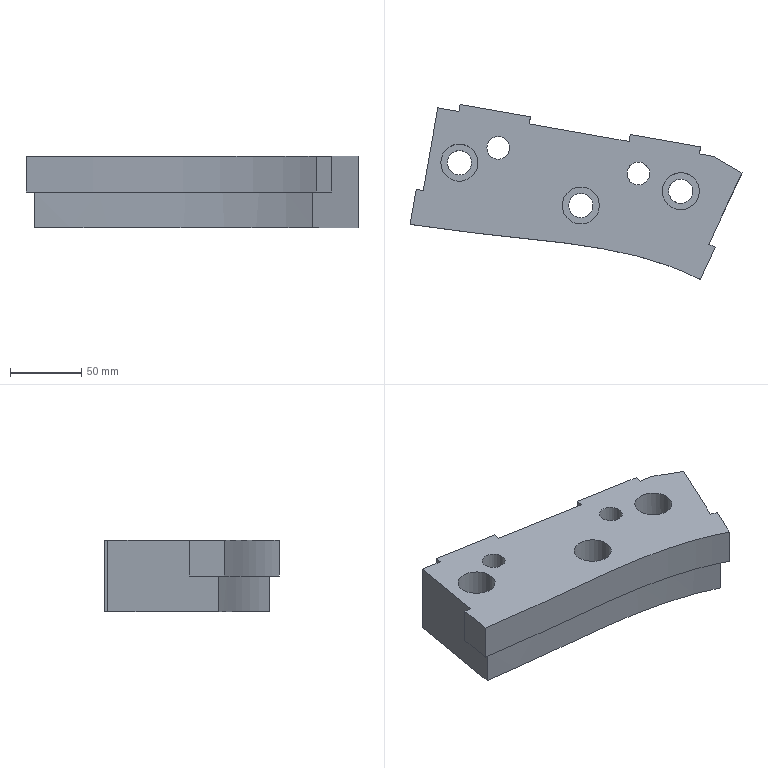Part | NX | features solid 2 | 1 solid | 32 faces | box 232.476 x 122.521 x 50 mm | volume 761001 mm3 | plane 22 | cylinder 8 | spline 2 | commonest cylinder face diameters 17 x3 26 x3 16 x2
STEP:
#1=CARTESIAN_POINT('',(-172.568,-241.894,-25.));
#2=VERTEX_POINT('',#1);
#3=CARTESIAN_POINT('',(-183.133,-264.552,-25.));
#4=VERTEX_POINT('',#3);
#5=CARTESIAN_POINT('',(-183.133,-264.552,-25.));
#6=DIRECTION('',(-0.4226,-0.9063,0.));
#7=VECTOR('',#6,1000.);
#8=LINE('',#5,#7);
#9=EDGE_CURVE('',#2,#4,#8,.T.);
#10=ORIENTED_EDGE('',*,*,#9,.F.);
#11=CARTESIAN_POINT('',(-172.568,-241.894,0.));
#12=VERTEX_POINT('',#11);
#13=CARTESIAN_POINT('',(-172.568,-241.894,-50.));
#14=DIRECTION('',(0.,0.,1.));
#15=VECTOR('',#14,1000.);
#16=LINE('',#13,#15);
#17=EDGE_CURVE('',#2,#12,#16,.T.);
#18=ORIENTED_EDGE('',*,*,#17,.T.);
#19=CARTESIAN_POINT('',(-183.133,-264.552,0.));
#20=VERTEX_POINT('',#19);
#21=CARTESIAN_POINT('',(-183.133,-264.552,0.));
#22=DIRECTION('',(0.4226,0.9063,0.));
#23=VECTOR('',#22,1000.);
#24=LINE('',#21,#23);
#25=EDGE_CURVE('',#20,#12,#24,.T.);
#26=ORIENTED_EDGE('',*,*,#25,.F.);
#27=CARTESIAN_POINT('',(-183.133,-264.552,-50.));
#28=DIRECTION('',(0.,0.,1.));
#29=VECTOR('',#28,1000.);
#30=LINE('',#27,#29);
#31=EDGE_CURVE('',#4,#20,#30,.T.);
#32=ORIENTED_EDGE('',*,*,#31,.F.);
#33=EDGE_LOOP('',(#10,#18,#26,#32));
#34=FACE_BOUND('',#33,.T.);
#35=CARTESIAN_POINT('',(-183.133,-264.552,-50.));
#36=DIRECTION('',(0.9063,-0.4226,0.));
#37=DIRECTION('',(0.4226,0.9063,0.));
#38=AXIS2_PLACEMENT_3D('',#35,#36,#37);
#39=PLANE('',#38);
#40=ADVANCED_FACE('',(#34),#39,.T.);
#41=CARTESIAN_POINT('',(-332.523,-172.421,0.));
#42=VERTEX_POINT('',#41);
#43=CARTESIAN_POINT('',(-324.523,-172.421,0.));
#44=DIRECTION('',(0.,0.,-1.));
#45=DIRECTION('',(-1.,0.,0.));
#46=AXIS2_PLACEMENT_3D('',#43,#44,#45);
#47=CIRCLE('',#46,8.);
#48=EDGE_CURVE('',#42,#42,#47,.T.);
#49=ORIENTED_EDGE('',*,*,#48,.T.);
#50=EDGE_LOOP('',(#49));
#51=FACE_BOUND('',#50,.T.);
#52=CARTESIAN_POINT('',(-234.374,-190.368,0.));
#53=VERTEX_POINT('',#52);
#54=CARTESIAN_POINT('',(-226.374,-190.368,0.));
#55=DIRECTION('',(0.,0.,-1.));
#56=DIRECTION('',(-1.,0.,0.));
#57=AXIS2_PLACEMENT_3D('',#54,#55,#56);
#58=CIRCLE('',#57,8.);
#59=EDGE_CURVE('',#53,#53,#58,.T.);
#60=ORIENTED_EDGE('',*,*,#59,.T.);
#61=EDGE_LOOP('',(#60));
#62=FACE_BOUND('',#61,.T.);
#63=CARTESIAN_POINT('',(-364.729,-182.741,0.));
#64=VERTEX_POINT('',#63);
#65=CARTESIAN_POINT('',(-351.729,-182.741,0.));
#66=DIRECTION('',(0.,0.,-1.));
#67=DIRECTION('',(-1.,0.,0.));
#68=AXIS2_PLACEMENT_3D('',#65,#66,#67);
#69=CIRCLE('',#68,13.);
#70=EDGE_CURVE('',#64,#64,#69,.T.);
#71=ORIENTED_EDGE('',*,*,#70,.T.);
#72=EDGE_LOOP('',(#71));
#73=FACE_BOUND('',#72,.T.);
#74=CARTESIAN_POINT('',(-279.729,-212.741,0.));
#75=VERTEX_POINT('',#74);
#76=CARTESIAN_POINT('',(-266.729,-212.741,0.));
#77=DIRECTION('',(0.,0.,-1.));
#78=DIRECTION('',(-1.,0.,0.));
#79=AXIS2_PLACEMENT_3D('',#76,#77,#78);
#80=CIRCLE('',#79,13.);
#81=EDGE_CURVE('',#75,#75,#80,.T.);
#82=ORIENTED_EDGE('',*,*,#81,.T.);
#83=EDGE_LOOP('',(#82));
#84=FACE_BOUND('',#83,.T.);
#85=CARTESIAN_POINT('',(-209.729,-202.741,0.));
#86=VERTEX_POINT('',#85);
#87=CARTESIAN_POINT('',(-196.729,-202.741,0.));
#88=DIRECTION('',(0.,0.,-1.));
#89=DIRECTION('',(-1.,0.,0.));
#90=AXIS2_PLACEMENT_3D('',#87,#88,#89);
#91=CIRCLE('',#90,13.);
#92=EDGE_CURVE('',#86,#86,#91,.T.);
#93=ORIENTED_EDGE('',*,*,#92,.T.);
#94=EDGE_LOOP('',(#93));
#95=FACE_BOUND('',#94,.T.);
#96=CARTESIAN_POINT('',(-177.099,-239.781,0.));
#97=VERTEX_POINT('',#96);
#98=CARTESIAN_POINT('',(-177.099,-239.781,0.));
#99=DIRECTION('',(0.9063,-0.4226,0.));
#100=VECTOR('',#99,1000.);
#101=LINE('',#98,#100);
#102=EDGE_CURVE('',#97,#12,#101,.T.);
#103=ORIENTED_EDGE('',*,*,#102,.F.);
#104=CARTESIAN_POINT('',(-153.848,-189.919,0.));
#105=VERTEX_POINT('',#104);
#106=CARTESIAN_POINT('',(-187.665,-262.438,0.));
#107=DIRECTION('',(0.4226,0.9063,0.));
#108=VECTOR('',#107,1000.);
#109=LINE('',#106,#108);
#110=EDGE_CURVE('',#97,#105,#109,.T.);
#111=ORIENTED_EDGE('',*,*,#110,.T.);
#112=CARTESIAN_POINT('',(-173.828,-178.383,0.));
#113=VERTEX_POINT('',#112);
#114=CARTESIAN_POINT('',(-229.835,-146.048,0.));
#115=DIRECTION('',(0.866,-0.5,0.));
#116=VECTOR('',#115,1000.);
#117=LINE('',#114,#116);
#118=EDGE_CURVE('',#113,#105,#117,.T.);
#119=ORIENTED_EDGE('',*,*,#118,.F.);
#120=CARTESIAN_POINT('',(-183.676,-176.647,0.));
#121=VERTEX_POINT('',#120);
#122=CARTESIAN_POINT('',(-371.767,-143.481,0.));
#123=DIRECTION('',(0.9848,-0.1736,0.));
#124=VECTOR('',#123,1000.);
#125=LINE('',#122,#124);
#126=EDGE_CURVE('',#121,#113,#125,.T.);
#127=ORIENTED_EDGE('',*,*,#126,.F.);
#128=CARTESIAN_POINT('',(-182.808,-171.723,0.));
#129=VERTEX_POINT('',#128);
#130=CARTESIAN_POINT('',(-183.676,-176.647,0.));
#131=DIRECTION('',(0.1736,0.9848,0.));
#132=VECTOR('',#131,1000.);
#133=LINE('',#130,#132);
#134=EDGE_CURVE('',#121,#129,#133,.T.);
#135=ORIENTED_EDGE('',*,*,#134,.T.);
#136=CARTESIAN_POINT('',(-232.048,-163.04,0.));
#137=VERTEX_POINT('',#136);
#138=CARTESIAN_POINT('',(-370.899,-138.557,0.));
#139=DIRECTION('',(0.9848,-0.1736,0.));
#140=VECTOR('',#139,1000.);
#141=LINE('',#138,#140);
#142=EDGE_CURVE('',#137,#129,#141,.T.);
#143=ORIENTED_EDGE('',*,*,#142,.F.);
#144=CARTESIAN_POINT('',(-232.916,-167.964,0.));
#145=VERTEX_POINT('',#144);
#146=CARTESIAN_POINT('',(-232.916,-167.964,0.));
#147=DIRECTION('',(0.1736,0.9848,0.));
#148=VECTOR('',#147,1000.);
#149=LINE('',#146,#148);
#150=EDGE_CURVE('',#145,#137,#149,.T.);
#151=ORIENTED_EDGE('',*,*,#150,.F.);
#152=CARTESIAN_POINT('',(-302.831,-155.637,0.));
#153=VERTEX_POINT('',#152);
#154=CARTESIAN_POINT('',(-371.767,-143.481,0.));
#155=DIRECTION('',(0.9848,-0.1736,0.));
#156=VECTOR('',#155,1000.);
#157=LINE('',#154,#156);
#158=EDGE_CURVE('',#153,#145,#157,.T.);
#159=ORIENTED_EDGE('',*,*,#158,.F.);
#160=CARTESIAN_POINT('',(-301.962,-150.713,0.));
#161=VERTEX_POINT('',#160);
#162=CARTESIAN_POINT('',(-302.831,-155.637,0.));
#163=DIRECTION('',(0.1736,0.9848,0.));
#164=VECTOR('',#163,1000.);
#165=LINE('',#162,#164);
#166=EDGE_CURVE('',#153,#161,#165,.T.);
#167=ORIENTED_EDGE('',*,*,#166,.T.);
#168=CARTESIAN_POINT('',(-351.203,-142.03,0.));
#169=VERTEX_POINT('',#168);
#170=CARTESIAN_POINT('',(-504.826,-114.942,0.));
#171=DIRECTION('',(0.9848,-0.1736,0.));
#172=VECTOR('',#171,1000.);
#173=LINE('',#170,#172);
#174=EDGE_CURVE('',#169,#161,#173,.T.);
#175=ORIENTED_EDGE('',*,*,#174,.F.);
#176=CARTESIAN_POINT('',(-352.071,-146.954,0.));
#177=VERTEX_POINT('',#176);
#178=CARTESIAN_POINT('',(-352.071,-146.954,0.));
#179=DIRECTION('',(0.1736,0.9848,0.));
#180=VECTOR('',#179,1000.);
#181=LINE('',#178,#180);
#182=EDGE_CURVE('',#177,#169,#181,.T.);
#183=ORIENTED_EDGE('',*,*,#182,.F.);
#184=CARTESIAN_POINT('',(-366.843,-144.35,0.));
#185=VERTEX_POINT('',#184);
#186=CARTESIAN_POINT('',(-371.767,-143.481,0.));
#187=DIRECTION('',(0.9848,-0.1736,0.));
#188=VECTOR('',#187,1000.);
#189=LINE('',#186,#188);
#190=EDGE_CURVE('',#185,#177,#189,.T.);
#191=ORIENTED_EDGE('',*,*,#190,.F.);
#192=CARTESIAN_POINT('',(-377.059,-202.288,0.));
#193=VERTEX_POINT('',#192);
#194=CARTESIAN_POINT('',(-381.401,-226.908,0.));
#195=DIRECTION('',(0.1736,0.9848,0.));
#196=VECTOR('',#195,1000.);
#197=LINE('',#194,#196);
#198=EDGE_CURVE('',#193,#185,#197,.T.);
#199=ORIENTED_EDGE('',*,*,#198,.F.);
#200=CARTESIAN_POINT('',(-381.983,-201.42,0.));
#201=VERTEX_POINT('',#200);
#202=CARTESIAN_POINT('',(-377.059,-202.288,0.));
#203=DIRECTION('',(-0.9848,0.1736,0.));
#204=VECTOR('',#203,1000.);
#205=LINE('',#202,#204);
#206=EDGE_CURVE('',#193,#201,#205,.T.);
#207=ORIENTED_EDGE('',*,*,#206,.T.);
#208=CARTESIAN_POINT('',(-386.325,-226.04,0.));
#209=VERTEX_POINT('',#208);
#210=CARTESIAN_POINT('',(-386.325,-226.04,0.));
#211=DIRECTION('',(0.1736,0.9848,0.));
#212=VECTOR('',#211,1000.);
#213=LINE('',#210,#212);
#214=EDGE_CURVE('',#209,#201,#213,.T.);
#215=ORIENTED_EDGE('',*,*,#214,.F.);
#216=CARTESIAN_POINT('',(-386.325,-226.04,0.));
#217=CARTESIAN_POINT('',(-385.988,-226.092,0.));
#218=CARTESIAN_POINT('',(-371.935,-228.253,0.));
#219=CARTESIAN_POINT('',(-344.075,-231.948,0.));
#220=CARTESIAN_POINT('',(-302.639,-236.064,0.));
#221=CARTESIAN_POINT('',(-261.264,-240.795,0.));
#222=CARTESIAN_POINT('',(-220.785,-248.799,0.));
#223=CARTESIAN_POINT('',(-195.074,-258.417,0.));
#224=CARTESIAN_POINT('',(-183.133,-264.552,0.));
#225=B_SPLINE_CURVE_WITH_KNOTS('',3,(#216,#217,#218,#219,#220,#221,#222,#223,#224),.UNSPECIFIED.,.F.,.F.,(4,1,1,1,1,1,4),(0.,0.004908,0.2052,0.4055,0.6058,0.8062,1.),.UNSPECIFIED.);
#226=EDGE_CURVE('',#209,#20,#225,.T.);
#227=ORIENTED_EDGE('',*,*,#226,.T.);
#228=ORIENTED_EDGE('',*,*,#25,.T.);
#229=EDGE_LOOP('',(#103,#111,#119,#127,#135,#143,#151,#159,#167,#175,#183,#191,#199,#207,#215,#227,#228));
#230=FACE_BOUND('',#229,.T.);
#231=CARTESIAN_POINT('',(-283.137,-238.369,0.));
#232=DIRECTION('',(0.,0.,-1.));
#233=DIRECTION('',(-1.,0.,0.));
#234=AXIS2_PLACEMENT_3D('',#231,#232,#233);
#235=PLANE('',#234);
#236=ADVANCED_FACE('',(#51,#62,#73,#84,#95,#230),#235,.F.);
#237=CARTESIAN_POINT('',(-177.099,-239.781,-25.));
#238=VERTEX_POINT('',#237);
#239=CARTESIAN_POINT('',(-177.099,-239.781,-25.));
#240=DIRECTION('',(0.9063,-0.4226,0.));
#241=VECTOR('',#240,1000.);
#242=LINE('',#239,#241);
#243=EDGE_CURVE('',#238,#2,#242,.T.);
#244=ORIENTED_EDGE('',*,*,#243,.T.);
#245=ORIENTED_EDGE('',*,*,#9,.T.);
#246=CARTESIAN_POINT('',(-386.325,-226.04,-25.));
#247=VERTEX_POINT('',#246);
#248=CARTESIAN_POINT('',(-386.325,-226.04,-25.));
#249=CARTESIAN_POINT('',(-385.988,-226.092,-25.));
#250=CARTESIAN_POINT('',(-371.935,-228.253,-25.));
#251=CARTESIAN_POINT('',(-344.075,-231.948,-25.));
#252=CARTESIAN_POINT('',(-302.639,-236.064,-25.));
#253=CARTESIAN_POINT('',(-261.264,-240.795,-25.));
#254=CARTESIAN_POINT('',(-220.785,-248.799,-25.));
#255=CARTESIAN_POINT('',(-195.074,-258.417,-25.));
#256=CARTESIAN_POINT('',(-183.133,-264.552,-25.));
#257=B_SPLINE_CURVE_WITH_KNOTS('',3,(#248,#249,#250,#251,#252,#253,#254,#255,#256),.UNSPECIFIED.,.F.,.F.,(4,1,1,1,1,1,4),(0.,0.004908,0.2052,0.4055,0.6058,0.8062,1.),.UNSPECIFIED.);
#258=EDGE_CURVE('',#4,#247,#257,.F.);
#259=ORIENTED_EDGE('',*,*,#258,.T.);
#260=CARTESIAN_POINT('',(-381.983,-201.42,-25.));
#261=VERTEX_POINT('',#260);
#262=CARTESIAN_POINT('',(-386.325,-226.04,-25.));
#263=DIRECTION('',(-0.1736,-0.9848,0.));
#264=VECTOR('',#263,1000.);
#265=LINE('',#262,#264);
#266=EDGE_CURVE('',#261,#247,#265,.T.);
#267=ORIENTED_EDGE('',*,*,#266,.F.);
#268=CARTESIAN_POINT('',(-377.059,-202.288,-25.));
#269=VERTEX_POINT('',#268);
#270=CARTESIAN_POINT('',(-377.059,-202.288,-25.));
#271=DIRECTION('',(-0.9848,0.1736,0.));
#272=VECTOR('',#271,1000.);
#273=LINE('',#270,#272);
#274=EDGE_CURVE('',#269,#261,#273,.T.);
#275=ORIENTED_EDGE('',*,*,#274,.F.);
#276=CARTESIAN_POINT('',(-380.511,-221.865,-25.));
#277=VERTEX_POINT('',#276);
#278=CARTESIAN_POINT('',(-381.401,-226.908,-25.));
#279=DIRECTION('',(-0.1736,-0.9848,0.));
#280=VECTOR('',#279,1000.);
#281=LINE('',#278,#280);
#282=EDGE_CURVE('',#277,#269,#281,.F.);
#283=ORIENTED_EDGE('',*,*,#282,.F.);
#284=CARTESIAN_POINT('',(-185.501,-257.798,-25.));
#285=VERTEX_POINT('',#284);
#286=CARTESIAN_POINT('',(-380.511,-221.865,-25.));
#287=CARTESIAN_POINT('',(-364.297,-224.285,-25.));
#288=CARTESIAN_POINT('',(-331.761,-228.294,-25.));
#289=CARTESIAN_POINT('',(-282.53,-232.98,-25.));
#290=CARTESIAN_POINT('',(-233.079,-240.247,-25.));
#291=CARTESIAN_POINT('',(-200.769,-250.502,-25.));
#292=CARTESIAN_POINT('',(-185.501,-257.798,-25.));
#293=B_SPLINE_CURVE_WITH_KNOTS('',3,(#286,#287,#288,#289,#290,#291,#292),.UNSPECIFIED.,.F.,.F.,(4,1,1,1,4),(0.0247,0.2624,0.5002,0.7379,0.9757),.UNSPECIFIED.);
#294=EDGE_CURVE('',#277,#285,#293,.T.);
#295=ORIENTED_EDGE('',*,*,#294,.T.);
#296=CARTESIAN_POINT('',(-187.665,-262.438,-25.));
#297=DIRECTION('',(-0.4226,-0.9063,0.));
#298=VECTOR('',#297,1000.);
#299=LINE('',#296,#298);
#300=EDGE_CURVE('',#285,#238,#299,.F.);
#301=ORIENTED_EDGE('',*,*,#300,.T.);
#302=EDGE_LOOP('',(#244,#245,#259,#267,#275,#283,#295,#301));
#303=FACE_BOUND('',#302,.T.);
#304=CARTESIAN_POINT('',(-386.325,-226.04,-25.));
#305=DIRECTION('',(0.,0.,1.));
#306=DIRECTION('',(1.,0.,0.));
#307=AXIS2_PLACEMENT_3D('',#304,#305,#306);
#308=PLANE('',#307);
#309=ADVANCED_FACE('',(#303),#308,.F.);
#310=ORIENTED_EDGE('',*,*,#118,.T.);
#311=CARTESIAN_POINT('',(-153.848,-189.919,-50.));
#312=VERTEX_POINT('',#311);
#313=CARTESIAN_POINT('',(-153.848,-189.919,-25.));
#314=DIRECTION('',(0.,0.,-1.));
#315=VECTOR('',#314,1000.);
#316=LINE('',#313,#315);
#317=EDGE_CURVE('',#105,#312,#316,.T.);
#318=ORIENTED_EDGE('',*,*,#317,.T.);
#319=CARTESIAN_POINT('',(-173.828,-178.383,-50.));
#320=VERTEX_POINT('',#319);
#321=CARTESIAN_POINT('',(-229.835,-146.048,-50.));
#322=DIRECTION('',(0.866,-0.5,0.));
#323=VECTOR('',#322,1000.);
#324=LINE('',#321,#323);
#325=EDGE_CURVE('',#320,#312,#324,.T.);
#326=ORIENTED_EDGE('',*,*,#325,.F.);
#327=CARTESIAN_POINT('',(-173.828,-178.383,-50.));
#328=DIRECTION('',(0.,0.,1.));
#329=VECTOR('',#328,1000.);
#330=LINE('',#327,#329);
#331=EDGE_CURVE('',#320,#113,#330,.T.);
#332=ORIENTED_EDGE('',*,*,#331,.T.);
#333=EDGE_LOOP('',(#310,#318,#326,#332));
#334=FACE_BOUND('',#333,.T.);
#335=CARTESIAN_POINT('',(32.129,-297.293,0.));
#336=DIRECTION('',(0.5,0.866,0.));
#337=DIRECTION('',(-0.866,0.5,0.));
#338=AXIS2_PLACEMENT_3D('',#335,#336,#337);
#339=PLANE('',#338);
#340=ADVANCED_FACE('',(#334),#339,.T.);
#341=CARTESIAN_POINT('',(-302.831,-155.637,-50.));
#342=VERTEX_POINT('',#341);
#343=CARTESIAN_POINT('',(-302.831,-155.637,-50.));
#344=DIRECTION('',(0.,0.,1.));
#345=VECTOR('',#344,1000.);
#346=LINE('',#343,#345);
#347=EDGE_CURVE('',#342,#153,#346,.T.);
#348=ORIENTED_EDGE('',*,*,#347,.T.);
#349=ORIENTED_EDGE('',*,*,#158,.T.);
#350=CARTESIAN_POINT('',(-232.916,-167.964,-50.));
#351=VERTEX_POINT('',#350);
#352=CARTESIAN_POINT('',(-232.916,-167.964,-50.));
#353=DIRECTION('',(0.,0.,-1.));
#354=VECTOR('',#353,1000.);
#355=LINE('',#352,#354);
#356=EDGE_CURVE('',#145,#351,#355,.T.);
#357=ORIENTED_EDGE('',*,*,#356,.T.);
#358=CARTESIAN_POINT('',(-371.767,-143.481,-50.));
#359=DIRECTION('',(0.9848,-0.1736,0.));
#360=VECTOR('',#359,1000.);
#361=LINE('',#358,#360);
#362=EDGE_CURVE('',#342,#351,#361,.T.);
#363=ORIENTED_EDGE('',*,*,#362,.F.);
#364=EDGE_LOOP('',(#348,#349,#357,#363));
#365=FACE_BOUND('',#364,.T.);
#366=CARTESIAN_POINT('',(-371.767,-143.481,-50.));
#367=DIRECTION('',(-0.1736,-0.9848,0.));
#368=DIRECTION('',(0.9848,-0.1736,0.));
#369=AXIS2_PLACEMENT_3D('',#366,#367,#368);
#370=PLANE('',#369);
#371=ADVANCED_FACE('',(#365),#370,.F.);
#372=CARTESIAN_POINT('',(-366.843,-144.35,-50.));
#373=VERTEX_POINT('',#372);
#374=CARTESIAN_POINT('',(-366.843,-144.35,-50.));
#375=DIRECTION('',(0.,0.,-1.));
#376=VECTOR('',#375,1000.);
#377=LINE('',#374,#376);
#378=EDGE_CURVE('',#185,#373,#377,.T.);
#379=ORIENTED_EDGE('',*,*,#378,.F.);
#380=ORIENTED_EDGE('',*,*,#190,.T.);
#381=CARTESIAN_POINT('',(-352.071,-146.954,-50.));
#382=VERTEX_POINT('',#381);
#383=CARTESIAN_POINT('',(-352.071,-146.954,-50.));
#384=DIRECTION('',(0.,0.,-1.));
#385=VECTOR('',#384,1000.);
#386=LINE('',#383,#385);
#387=EDGE_CURVE('',#177,#382,#386,.T.);
#388=ORIENTED_EDGE('',*,*,#387,.T.);
#389=CARTESIAN_POINT('',(-371.767,-143.481,-50.));
#390=DIRECTION('',(0.9848,-0.1736,0.));
#391=VECTOR('',#390,1000.);
#392=LINE('',#389,#391);
#393=EDGE_CURVE('',#373,#382,#392,.T.);
#394=ORIENTED_EDGE('',*,*,#393,.F.);
#395=EDGE_LOOP('',(#379,#380,#388,#394));
#396=FACE_BOUND('',#395,.T.);
#397=CARTESIAN_POINT('',(-371.767,-143.481,-50.));
#398=DIRECTION('',(-0.1736,-0.9848,0.));
#399=DIRECTION('',(0.9848,-0.1736,0.));
#400=AXIS2_PLACEMENT_3D('',#397,#398,#399);
#401=PLANE('',#400);
#402=ADVANCED_FACE('',(#396),#401,.F.);
#403=CARTESIAN_POINT('',(-183.676,-176.647,-50.));
#404=VERTEX_POINT('',#403);
#405=CARTESIAN_POINT('',(-183.676,-176.647,-50.));
#406=DIRECTION('',(0.,0.,1.));
#407=VECTOR('',#406,1000.);
#408=LINE('',#405,#407);
#409=EDGE_CURVE('',#404,#121,#408,.T.);
#410=ORIENTED_EDGE('',*,*,#409,.T.);
#411=ORIENTED_EDGE('',*,*,#126,.T.);
#412=ORIENTED_EDGE('',*,*,#331,.F.);
#413=CARTESIAN_POINT('',(-371.767,-143.481,-50.));
#414=DIRECTION('',(0.9848,-0.1736,0.));
#415=VECTOR('',#414,1000.);
#416=LINE('',#413,#415);
#417=EDGE_CURVE('',#404,#320,#416,.T.);
#418=ORIENTED_EDGE('',*,*,#417,.F.);
#419=EDGE_LOOP('',(#410,#411,#412,#418));
#420=FACE_BOUND('',#419,.T.);
#421=CARTESIAN_POINT('',(-371.767,-143.481,-50.));
#422=DIRECTION('',(-0.1736,-0.9848,0.));
#423=DIRECTION('',(0.9848,-0.1736,0.));
#424=AXIS2_PLACEMENT_3D('',#421,#422,#423);
#425=PLANE('',#424);
#426=ADVANCED_FACE('',(#420),#425,.F.);
#427=CARTESIAN_POINT('',(-332.523,-172.421,-50.));
#428=VERTEX_POINT('',#427);
#429=CARTESIAN_POINT('',(-324.523,-172.421,-50.));
#430=DIRECTION('',(0.,0.,-1.));
#431=DIRECTION('',(-1.,0.,0.));
#432=AXIS2_PLACEMENT_3D('',#429,#430,#431);
#433=CIRCLE('',#432,8.);
#434=EDGE_CURVE('',#428,#428,#433,.T.);
#435=ORIENTED_EDGE('',*,*,#434,.F.);
#436=EDGE_LOOP('',(#435));
#437=FACE_BOUND('',#436,.T.);
#438=CARTESIAN_POINT('',(-234.374,-190.368,-50.));
#439=VERTEX_POINT('',#438);
#440=CARTESIAN_POINT('',(-226.374,-190.368,-50.));
#441=DIRECTION('',(0.,0.,-1.));
#442=DIRECTION('',(-1.,0.,0.));
#443=AXIS2_PLACEMENT_3D('',#440,#441,#442);
#444=CIRCLE('',#443,8.);
#445=EDGE_CURVE('',#439,#439,#444,.T.);
#446=ORIENTED_EDGE('',*,*,#445,.F.);
#447=EDGE_LOOP('',(#446));
#448=FACE_BOUND('',#447,.T.);
#449=CARTESIAN_POINT('',(-205.229,-202.741,-50.));
#450=VERTEX_POINT('',#449);
#451=CARTESIAN_POINT('',(-196.729,-202.741,-50.));
#452=DIRECTION('',(0.,0.,-1.));
#453=DIRECTION('',(-1.,0.,0.));
#454=AXIS2_PLACEMENT_3D('',#451,#452,#453);
#455=CIRCLE('',#454,8.5);
#456=EDGE_CURVE('',#450,#450,#455,.T.);
#457=ORIENTED_EDGE('',*,*,#456,.F.);
#458=EDGE_LOOP('',(#457));
#459=FACE_BOUND('',#458,.T.);
#460=CARTESIAN_POINT('',(-275.229,-212.741,-50.));
#461=VERTEX_POINT('',#460);
#462=CARTESIAN_POINT('',(-266.729,-212.741,-50.));
#463=DIRECTION('',(0.,0.,-1.));
#464=DIRECTION('',(-1.,0.,0.));
#465=AXIS2_PLACEMENT_3D('',#462,#463,#464);
#466=CIRCLE('',#465,8.5);
#467=EDGE_CURVE('',#461,#461,#466,.T.);
#468=ORIENTED_EDGE('',*,*,#467,.F.);
#469=EDGE_LOOP('',(#468));
#470=FACE_BOUND('',#469,.T.);
#471=CARTESIAN_POINT('',(-360.229,-182.741,-50.));
#472=VERTEX_POINT('',#471);
#473=CARTESIAN_POINT('',(-351.729,-182.741,-50.));
#474=DIRECTION('',(0.,0.,-1.));
#475=DIRECTION('',(-1.,0.,0.));
#476=AXIS2_PLACEMENT_3D('',#473,#474,#475);
#477=CIRCLE('',#476,8.5);
#478=EDGE_CURVE('',#472,#472,#477,.T.);
#479=ORIENTED_EDGE('',*,*,#478,.F.);
#480=EDGE_LOOP('',(#479));
#481=FACE_BOUND('',#480,.T.);
#482=ORIENTED_EDGE('',*,*,#393,.T.);
#483=CARTESIAN_POINT('',(-351.203,-142.03,-50.));
#484=VERTEX_POINT('',#483);
#485=CARTESIAN_POINT('',(-352.071,-146.954,-50.));
#486=DIRECTION('',(0.1736,0.9848,0.));
#487=VECTOR('',#486,1000.);
#488=LINE('',#485,#487);
#489=EDGE_CURVE('',#382,#484,#488,.T.);
#490=ORIENTED_EDGE('',*,*,#489,.T.);
#491=CARTESIAN_POINT('',(-301.962,-150.713,-50.));
#492=VERTEX_POINT('',#491);
#493=CARTESIAN_POINT('',(-504.826,-114.942,-50.));
#494=DIRECTION('',(0.9848,-0.1736,0.));
#495=VECTOR('',#494,1000.);
#496=LINE('',#493,#495);
#497=EDGE_CURVE('',#484,#492,#496,.T.);
#498=ORIENTED_EDGE('',*,*,#497,.T.);
#499=CARTESIAN_POINT('',(-302.831,-155.637,-50.));
#500=DIRECTION('',(0.1736,0.9848,0.));
#501=VECTOR('',#500,1000.);
#502=LINE('',#499,#501);
#503=EDGE_CURVE('',#342,#492,#502,.T.);
#504=ORIENTED_EDGE('',*,*,#503,.F.);
#505=ORIENTED_EDGE('',*,*,#362,.T.);
#506=CARTESIAN_POINT('',(-232.048,-163.04,-50.));
#507=VERTEX_POINT('',#506);
#508=CARTESIAN_POINT('',(-232.916,-167.964,-50.));
#509=DIRECTION('',(0.1736,0.9848,0.));
#510=VECTOR('',#509,1000.);
#511=LINE('',#508,#510);
#512=EDGE_CURVE('',#351,#507,#511,.T.);
#513=ORIENTED_EDGE('',*,*,#512,.T.);
#514=CARTESIAN_POINT('',(-182.808,-171.723,-50.));
#515=VERTEX_POINT('',#514);
#516=CARTESIAN_POINT('',(-370.899,-138.557,-50.));
#517=DIRECTION('',(0.9848,-0.1736,0.));
#518=VECTOR('',#517,1000.);
#519=LINE('',#516,#518);
#520=EDGE_CURVE('',#507,#515,#519,.T.);
#521=ORIENTED_EDGE('',*,*,#520,.T.);
#522=CARTESIAN_POINT('',(-183.676,-176.647,-50.));
#523=DIRECTION('',(0.1736,0.9848,0.));
#524=VECTOR('',#523,1000.);
#525=LINE('',#522,#524);
#526=EDGE_CURVE('',#404,#515,#525,.T.);
#527=ORIENTED_EDGE('',*,*,#526,.F.);
#528=ORIENTED_EDGE('',*,*,#417,.T.);
#529=ORIENTED_EDGE('',*,*,#325,.T.);
#530=CARTESIAN_POINT('',(-185.501,-257.798,-50.));
#531=VERTEX_POINT('',#530);
#532=CARTESIAN_POINT('',(-195.498,-279.236,-50.));
#533=DIRECTION('',(0.4226,0.9063,0.));
#534=VECTOR('',#533,1000.);
#535=LINE('',#532,#534);
#536=EDGE_CURVE('',#531,#312,#535,.T.);
#537=ORIENTED_EDGE('',*,*,#536,.F.);
#538=CARTESIAN_POINT('',(-380.511,-221.865,-50.));
#539=VERTEX_POINT('',#538);
#540=CARTESIAN_POINT('',(-185.501,-257.798,-50.));
#541=CARTESIAN_POINT('',(-188.943,-256.153,-50.));
#542=CARTESIAN_POINT('',(-196.057,-253.02,-50.));
#543=CARTESIAN_POINT('',(-205.525,-249.494,-50.));
#544=CARTESIAN_POINT('',(-213.444,-246.908,-50.));
#545=CARTESIAN_POINT('',(-219.56,-245.085,-50.));
#546=CARTESIAN_POINT('',(-224.788,-243.666,-50.));
#547=CARTESIAN_POINT('',(-228.548,-242.719,-50.));
#548=CARTESIAN_POINT('',(-230.68,-242.201,-50.));
#549=CARTESIAN_POINT('',(-232.396,-241.795,-50.));
#550=CARTESIAN_POINT('',(-233.719,-241.49,-50.));
#551=CARTESIAN_POINT('',(-235.645,-241.054,-50.));
#552=CARTESIAN_POINT('',(-239.001,-240.319,-50.));
#553=CARTESIAN_POINT('',(-243.982,-239.298,-50.));
#554=CARTESIAN_POINT('',(-249.135,-238.331,-50.));
#555=CARTESIAN_POINT('',(-252.875,-237.675,-50.));
#556=CARTESIAN_POINT('',(-255.001,-237.314,-50.));
#557=CARTESIAN_POINT('',(-256.723,-237.029,-50.));
#558=CARTESIAN_POINT('',(-258.029,-236.817,-50.));
#559=CARTESIAN_POINT('',(-259.948,-236.511,-50.));
#560=CARTESIAN_POINT('',(-263.303,-235.991,-50.));
#561=CARTESIAN_POINT('',(-267.323,-235.401,-50.));
#562=CARTESIAN_POINT('',(-271.486,-234.824,-50.));
#563=CARTESIAN_POINT('',(-274.691,-234.394,-50.));
#564=CARTESIAN_POINT('',(-277.413,-234.042,-50.));
#565=CARTESIAN_POINT('',(-279.378,-233.794,-50.));
#566=CARTESIAN_POINT('',(-280.471,-233.658,-50.));
#567=CARTESIAN_POINT('',(-281.408,-233.543,-50.));
#568=CARTESIAN_POINT('',(-281.919,-233.481,-50.));
#569=CARTESIAN_POINT('',(-282.768,-233.377,-50.));
#570=CARTESIAN_POINT('',(-284.222,-233.202,-50.));
#571=CARTESIAN_POINT('',(-286.447,-232.939,-50.));
#572=CARTESIAN_POINT('',(-289.279,-232.612,-50.));
#573=CARTESIAN_POINT('',(-292.293,-232.271,-50.));
#574=CARTESIAN_POINT('',(-295.483,-231.916,-50.));
#575=CARTESIAN_POINT('',(-298.29,-231.609,-50.));
#576=CARTESIAN_POINT('',(-300.624,-231.356,-50.));
#577=CARTESIAN_POINT('',(-302.12,-231.195,-50.));
#578=CARTESIAN_POINT('',(-303.338,-231.065,-50.));
#579=CARTESIAN_POINT('',(-304.266,-230.967,-50.));
#580=CARTESIAN_POINT('',(-305.039,-230.885,-50.));
#581=CARTESIAN_POINT('',(-305.604,-230.825,-50.));
#582=CARTESIAN_POINT('',(-305.897,-230.794,-50.));
#583=CARTESIAN_POINT('',(-306.206,-230.761,-50.));
#584=CARTESIAN_POINT('',(-306.179,-230.764,-50.));
#585=CARTESIAN_POINT('',(-306.269,-230.754,-50.));
#586=CARTESIAN_POINT('',(-306.387,-230.742,-50.));
#587=CARTESIAN_POINT('',(-306.631,-230.716,-50.));
#588=CARTESIAN_POINT('',(-306.988,-230.679,-50.));
#589=CARTESIAN_POINT('',(-307.569,-230.618,-50.));
#590=CARTESIAN_POINT('',(-308.484,-230.522,-50.));
#591=CARTESIAN_POINT('',(-309.885,-230.375,-50.));
#592=CARTESIAN_POINT('',(-311.587,-230.197,-50.));
#593=CARTESIAN_POINT('',(-313.597,-229.986,-50.));
#594=CARTESIAN_POINT('',(-315.512,-229.786,-50.));
#595=CARTESIAN_POINT('',(-317.008,-229.629,-50.));
#596=CARTESIAN_POINT('',(-317.865,-229.539,-50.));
#597=CARTESIAN_POINT('',(-318.629,-229.459,-50.));
#598=CARTESIAN_POINT('',(-319.019,-229.419,-50.));
#599=CARTESIAN_POINT('',(-319.661,-229.351,-50.));
#600=CARTESIAN_POINT('',(-320.707,-229.242,-50.));
#601=CARTESIAN_POINT('',(-322.181,-229.087,-50.));
#602=CARTESIAN_POINT('',(-323.854,-228.91,-50.));
#603=CARTESIAN_POINT('',(-325.448,-228.741,-50.));
#604=CARTESIAN_POINT('',(-326.957,-228.581,-50.));
#605=CARTESIAN_POINT('',(-328.39,-228.428,-50.));
#606=CARTESIAN_POINT('',(-329.497,-228.31,-50.));
#607=CARTESIAN_POINT('',(-330.382,-228.214,-50.));
#608=CARTESIAN_POINT('',(-330.914,-228.157,-50.));
#609=CARTESIAN_POINT('',(-331.852,-228.055,-50.));
#610=CARTESIAN_POINT('',(-332.948,-227.936,-50.));
#611=CARTESIAN_POINT('',(-334.908,-227.722,-50.));
#612=CARTESIAN_POINT('',(-337.597,-227.424,-50.));
#613=CARTESIAN_POINT('',(-340.724,-227.071,-50.));
#614=CARTESIAN_POINT('',(-343.715,-226.728,-50.));
#615=CARTESIAN_POINT('',(-345.905,-226.471,-50.));
#616=CARTESIAN_POINT('',(-347.273,-226.308,-50.));
#617=CARTESIAN_POINT('',(-348.307,-226.185,-50.));
#618=CARTESIAN_POINT('',(-350.179,-225.96,-50.));
#619=CARTESIAN_POINT('',(-352.808,-225.638,-50.));
#620=CARTESIAN_POINT('',(-357.009,-225.113,-50.));
#621=CARTESIAN_POINT('',(-362.211,-224.441,-50.));
#622=CARTESIAN_POINT('',(-370.443,-223.332,-50.));
#623=CARTESIAN_POINT('',(-376.512,-222.462,-50.));
#624=CARTESIAN_POINT('',(-380.511,-221.865,-50.));
#625=B_SPLINE_CURVE_WITH_KNOTS('',3,(#540,#541,#542,#543,#544,#545,#546,#547,#548,#549,#550,#551,#552,#553,#554,#555,#556,#557,#558,#559,#560,#561,#562,#563,#564,#565,#566,#567,#568,#569,#570,#571,#572,#573,#574,#575,#576,#577,#578,#579,#580,#581,#582,#583,#584,#585,#586,#587,#588,#589,#590,#591,#592,#593,#594,#595,#596,#597,#598,#599,#600,#601,#602,#603,#604,#605,#606,#607,#608,#609,#610,#611,#612,#613,#614,#615,#616,#617,#618,#619,#620,#621,#622,#623,#624),.UNSPECIFIED.,.F.,.F.,(4,1,1,1,1,1,1,1,1,1,1,1,1,1,1,1,1,1,1,1,1,1,1,1,1,1,1,1,1,1,1,1,1,1,1,1,1,1,1,1,1,1,1,1,1,1,1,1,1,1,1,1,1,1,1,1,1,1,1,1,1,1,1,1,1,1,1,1,1,1,1,1,1,1,1,1,1,1,1,1,1,1,4),(0.,0.0625,0.125,0.1562,0.1875,0.2188,0.2344,0.2422,0.25,0.2578,0.2656,0.2812,0.3125,0.3438,0.3594,0.3672,0.375,0.3828,0.3906,0.4062,0.4375,0.4531,0.4688,0.4844,0.4922,0.4961,0.5,0.5039,0.5078,0.5156,0.5312,0.5469,0.5625,0.5781,0.5938,0.6016,0.6094,0.6133,0.6172,0.6211,0.623,0.624,0.625,0.626,0.627,0.6289,0.6328,0.6367,0.6406,0.6484,0.6562,0.6641,0.6719,0.6797,0.6836,0.6855,0.6875,0.6895,0.6914,0.6953,0.7031,0.7109,0.7188,0.7266,0.7344,0.7422,0.7461,0.75,0.7539,0.7578,0.7656,0.7812,0.7969,0.8125,0.8281,0.832,0.8359,0.8438,0.8594,0.875,0.9062,0.9375,1.),.UNSPECIFIED.);
#626=EDGE_CURVE('',#539,#531,#625,.F.);
#627=ORIENTED_EDGE('',*,*,#626,.F.);
#628=CARTESIAN_POINT('',(-380.397,-221.22,-50.));
#629=DIRECTION('',(0.1736,0.9848,0.));
#630=VECTOR('',#629,1000.);
#631=LINE('',#628,#630);
#632=EDGE_CURVE('',#539,#373,#631,.T.);
#633=ORIENTED_EDGE('',*,*,#632,.T.);
#634=EDGE_LOOP('',(#482,#490,#498,#504,#505,#513,#521,#527,#528,#529,#537,#627,#633));
#635=FACE_BOUND('',#634,.T.);
#636=CARTESIAN_POINT('',(-283.137,-238.369,-50.));
#637=DIRECTION('',(0.,0.,-1.));
#638=DIRECTION('',(-1.,0.,0.));
#639=AXIS2_PLACEMENT_3D('',#636,#637,#638);
#640=PLANE('',#639);
#641=ADVANCED_FACE('',(#437,#448,#459,#470,#481,#635),#640,.T.);
#642=ORIENTED_EDGE('',*,*,#317,.F.);
#643=ORIENTED_EDGE('',*,*,#110,.F.);
#644=CARTESIAN_POINT('',(-177.099,-239.781,-50.));
#645=DIRECTION('',(0.,0.,1.));
#646=VECTOR('',#645,1000.);
#647=LINE('',#644,#646);
#648=EDGE_CURVE('',#238,#97,#647,.T.);
#649=ORIENTED_EDGE('',*,*,#648,.F.);
#650=ORIENTED_EDGE('',*,*,#300,.F.);
#651=CARTESIAN_POINT('',(-185.501,-257.798,-37.5));
#652=DIRECTION('',(0.,0.,-1.));
#653=VECTOR('',#652,1000.);
#654=LINE('',#651,#653);
#655=EDGE_CURVE('',#531,#285,#654,.F.);
#656=ORIENTED_EDGE('',*,*,#655,.F.);
#657=ORIENTED_EDGE('',*,*,#536,.T.);
#658=EDGE_LOOP('',(#642,#643,#649,#650,#656,#657));
#659=FACE_BOUND('',#658,.T.);
#660=CARTESIAN_POINT('',(-187.665,-262.438,-25.));
#661=DIRECTION('',(-0.9063,0.4226,0.));
#662=DIRECTION('',(-0.4226,-0.9063,0.));
#663=AXIS2_PLACEMENT_3D('',#660,#661,#662);
#664=PLANE('',#663);
#665=ADVANCED_FACE('',(#659),#664,.F.);
#666=CARTESIAN_POINT('',(-380.511,-221.865,-37.5));
#667=DIRECTION('',(0.,0.,-1.));
#668=VECTOR('',#667,1000.);
#669=LINE('',#666,#668);
#670=EDGE_CURVE('',#539,#277,#669,.F.);
#671=ORIENTED_EDGE('',*,*,#670,.F.);
#672=ORIENTED_EDGE('',*,*,#626,.T.);
#673=ORIENTED_EDGE('',*,*,#655,.T.);
#674=ORIENTED_EDGE('',*,*,#294,.F.);
#675=EDGE_LOOP('',(#671,#672,#673,#674));
#676=FACE_BOUND('',#675,.T.);
#677=CARTESIAN_POINT('',(-380.511,-221.865,-25.));
#678=CARTESIAN_POINT('',(-380.511,-221.865,-50.));
#679=CARTESIAN_POINT('',(-364.297,-224.285,-25.));
#680=CARTESIAN_POINT('',(-364.297,-224.285,-50.));
#681=CARTESIAN_POINT('',(-331.761,-228.294,-25.));
#682=CARTESIAN_POINT('',(-331.761,-228.294,-50.));
#683=CARTESIAN_POINT('',(-282.53,-232.98,-25.));
#684=CARTESIAN_POINT('',(-282.53,-232.98,-50.));
#685=CARTESIAN_POINT('',(-233.079,-240.247,-25.));
#686=CARTESIAN_POINT('',(-233.079,-240.247,-50.));
#687=CARTESIAN_POINT('',(-200.769,-250.502,-25.));
#688=CARTESIAN_POINT('',(-200.769,-250.502,-50.));
#689=CARTESIAN_POINT('',(-185.501,-257.798,-25.));
#690=CARTESIAN_POINT('',(-185.501,-257.798,-50.));
#691=B_SPLINE_SURFACE_WITH_KNOTS('',3,1,((#677,#678),(#679,#680),(#681,#682),(#683,#684),(#685,#686),(#687,#688),(#689,#690)),.SURF_OF_LINEAR_EXTRUSION.,.F.,.F.,.F.,(4,1,1,1,4),(2,2),(0.0247,0.2624,0.5002,0.7379,0.9757),(0.,1.),.UNSPECIFIED.);
#692=ADVANCED_FACE('',(#676),#691,.F.);
#693=ORIENTED_EDGE('',*,*,#214,.T.);
#694=CARTESIAN_POINT('',(-381.983,-201.42,-50.));
#695=DIRECTION('',(0.,0.,-1.));
#696=VECTOR('',#695,1000.);
#697=LINE('',#694,#696);
#698=EDGE_CURVE('',#201,#261,#697,.T.);
#699=ORIENTED_EDGE('',*,*,#698,.T.);
#700=ORIENTED_EDGE('',*,*,#266,.T.);
#701=CARTESIAN_POINT('',(-386.325,-226.04,-50.));
#702=DIRECTION('',(0.,0.,1.));
#703=VECTOR('',#702,1000.);
#704=LINE('',#701,#703);
#705=EDGE_CURVE('',#247,#209,#704,.T.);
#706=ORIENTED_EDGE('',*,*,#705,.T.);
#707=EDGE_LOOP('',(#693,#699,#700,#706));
#708=FACE_BOUND('',#707,.T.);
#709=CARTESIAN_POINT('',(-386.325,-226.04,-50.));
#710=DIRECTION('',(0.9848,-0.1736,0.));
#711=DIRECTION('',(0.1736,0.9848,0.));
#712=AXIS2_PLACEMENT_3D('',#709,#710,#711);
#713=PLANE('',#712);
#714=ADVANCED_FACE('',(#708),#713,.F.);
#715=ORIENTED_EDGE('',*,*,#258,.F.);
#716=ORIENTED_EDGE('',*,*,#31,.T.);
#717=ORIENTED_EDGE('',*,*,#226,.F.);
#718=ORIENTED_EDGE('',*,*,#705,.F.);
#719=EDGE_LOOP('',(#715,#716,#717,#718));
#720=FACE_BOUND('',#719,.T.);
#721=CARTESIAN_POINT('',(-386.325,-226.04,-25.));
#722=CARTESIAN_POINT('',(-386.325,-226.04,0.));
#723=CARTESIAN_POINT('',(-369.206,-228.681,-25.));
#724=CARTESIAN_POINT('',(-369.206,-228.681,0.));
#725=CARTESIAN_POINT('',(-334.829,-233.043,-25.));
#726=CARTESIAN_POINT('',(-334.829,-233.043,0.));
#727=CARTESIAN_POINT('',(-283.093,-237.907,-25.));
#728=CARTESIAN_POINT('',(-283.093,-237.907,0.));
#729=CARTESIAN_POINT('',(-231.62,-245.543,-25.));
#730=CARTESIAN_POINT('',(-231.62,-245.543,0.));
#731=CARTESIAN_POINT('',(-198.534,-256.64,-25.));
#732=CARTESIAN_POINT('',(-198.534,-256.64,0.));
#733=CARTESIAN_POINT('',(-183.133,-264.552,-25.));
#734=CARTESIAN_POINT('',(-183.133,-264.552,0.));
#735=B_SPLINE_SURFACE_WITH_KNOTS('',3,1,((#721,#722),(#723,#724),(#725,#726),(#727,#728),(#729,#730),(#731,#732),(#733,#734)),.SURF_OF_LINEAR_EXTRUSION.,.F.,.F.,.F.,(4,1,1,1,4),(2,2),(0.,0.25,0.5,0.75,1.),(0.,1.),.UNSPECIFIED.);
#736=ADVANCED_FACE('',(#720),#735,.T.);
#737=ORIENTED_EDGE('',*,*,#378,.T.);
#738=ORIENTED_EDGE('',*,*,#632,.F.);
#739=ORIENTED_EDGE('',*,*,#670,.T.);
#740=ORIENTED_EDGE('',*,*,#282,.T.);
#741=CARTESIAN_POINT('',(-377.059,-202.288,-50.));
#742=DIRECTION('',(0.,0.,1.));
#743=VECTOR('',#742,1000.);
#744=LINE('',#741,#743);
#745=EDGE_CURVE('',#269,#193,#744,.T.);
#746=ORIENTED_EDGE('',*,*,#745,.T.);
#747=ORIENTED_EDGE('',*,*,#198,.T.);
#748=EDGE_LOOP('',(#737,#738,#739,#740,#746,#747));
#749=FACE_BOUND('',#748,.T.);
#750=CARTESIAN_POINT('',(-381.401,-226.908,-25.));
#751=DIRECTION('',(-0.9848,0.1736,0.));
#752=DIRECTION('',(-0.1736,-0.9848,0.));
#753=AXIS2_PLACEMENT_3D('',#750,#751,#752);
#754=PLANE('',#753);
#755=ADVANCED_FACE('',(#749),#754,.T.);
#756=CARTESIAN_POINT('',(-196.729,-215.741,-25.));
#757=VERTEX_POINT('',#756);
#758=CARTESIAN_POINT('',(-196.729,-202.741,-25.));
#759=DIRECTION('',(0.,0.,1.));
#760=DIRECTION('',(0.,-1.,0.));
#761=AXIS2_PLACEMENT_3D('',#758,#759,#760);
#762=CIRCLE('',#761,13.);
#763=EDGE_CURVE('',#757,#757,#762,.T.);
#764=ORIENTED_EDGE('',*,*,#763,.F.);
#765=EDGE_LOOP('',(#764));
#766=FACE_BOUND('',#765,.T.);
#767=ORIENTED_EDGE('',*,*,#92,.F.);
#768=EDGE_LOOP('',(#767));
#769=FACE_BOUND('',#768,.T.);
#770=CARTESIAN_POINT('',(-196.729,-202.741,-25.));
#771=DIRECTION('',(0.,0.,1.));
#772=DIRECTION('',(0.,-1.,0.));
#773=AXIS2_PLACEMENT_3D('',#770,#771,#772);
#774=CYLINDRICAL_SURFACE('',#773,13.);
#775=ADVANCED_FACE('',(#766,#769),#774,.F.);
#776=ORIENTED_EDGE('',*,*,#456,.T.);
#777=EDGE_LOOP('',(#776));
#778=FACE_BOUND('',#777,.T.);
#779=CARTESIAN_POINT('',(-196.729,-194.241,-25.));
#780=VERTEX_POINT('',#779);
#781=CARTESIAN_POINT('',(-196.729,-202.741,-25.));
#782=DIRECTION('',(0.,0.,-1.));
#783=DIRECTION('',(0.,1.,0.));
#784=AXIS2_PLACEMENT_3D('',#781,#782,#783);
#785=CIRCLE('',#784,8.5);
#786=EDGE_CURVE('',#780,#780,#785,.F.);
#787=ORIENTED_EDGE('',*,*,#786,.T.);
#788=EDGE_LOOP('',(#787));
#789=FACE_BOUND('',#788,.T.);
#790=CARTESIAN_POINT('',(-196.729,-202.741,-75.));
#791=DIRECTION('',(0.,0.,1.));
#792=DIRECTION('',(0.,-1.,0.));
#793=AXIS2_PLACEMENT_3D('',#790,#791,#792);
#794=CYLINDRICAL_SURFACE('',#793,8.5);
#795=ADVANCED_FACE('',(#778,#789),#794,.F.);
#796=ORIENTED_EDGE('',*,*,#786,.F.);
#797=EDGE_LOOP('',(#796));
#798=FACE_BOUND('',#797,.T.);
#799=ORIENTED_EDGE('',*,*,#763,.T.);
#800=EDGE_LOOP('',(#799));
#801=FACE_BOUND('',#800,.T.);
#802=CARTESIAN_POINT('',(-196.729,-202.741,-25.));
#803=DIRECTION('',(0.,0.,-1.));
#804=DIRECTION('',(0.,1.,0.));
#805=AXIS2_PLACEMENT_3D('',#802,#803,#804);
#806=PLANE('',#805);
#807=ADVANCED_FACE('',(#798,#801),#806,.F.);
#808=CARTESIAN_POINT('',(-253.729,-212.741,-25.));
#809=VERTEX_POINT('',#808);
#810=CARTESIAN_POINT('',(-266.729,-212.741,-25.));
#811=DIRECTION('',(0.,0.,1.));
#812=DIRECTION('',(1.,0.,0.));
#813=AXIS2_PLACEMENT_3D('',#810,#811,#812);
#814=CIRCLE('',#813,13.);
#815=EDGE_CURVE('',#809,#809,#814,.T.);
#816=ORIENTED_EDGE('',*,*,#815,.F.);
#817=EDGE_LOOP('',(#816));
#818=FACE_BOUND('',#817,.T.);
#819=ORIENTED_EDGE('',*,*,#81,.F.);
#820=EDGE_LOOP('',(#819));
#821=FACE_BOUND('',#820,.T.);
#822=CARTESIAN_POINT('',(-266.729,-212.741,-25.));
#823=DIRECTION('',(0.,0.,1.));
#824=DIRECTION('',(1.,0.,0.));
#825=AXIS2_PLACEMENT_3D('',#822,#823,#824);
#826=CYLINDRICAL_SURFACE('',#825,13.);
#827=ADVANCED_FACE('',(#818,#821),#826,.F.);
#828=ORIENTED_EDGE('',*,*,#467,.T.);
#829=EDGE_LOOP('',(#828));
#830=FACE_BOUND('',#829,.T.);
#831=CARTESIAN_POINT('',(-275.229,-212.741,-25.));
#832=VERTEX_POINT('',#831);
#833=CARTESIAN_POINT('',(-266.729,-212.741,-25.));
#834=DIRECTION('',(0.,0.,-1.));
#835=DIRECTION('',(-1.,0.,0.));
#836=AXIS2_PLACEMENT_3D('',#833,#834,#835);
#837=CIRCLE('',#836,8.5);
#838=EDGE_CURVE('',#832,#832,#837,.F.);
#839=ORIENTED_EDGE('',*,*,#838,.T.);
#840=EDGE_LOOP('',(#839));
#841=FACE_BOUND('',#840,.T.);
#842=CARTESIAN_POINT('',(-266.729,-212.741,-75.));
#843=DIRECTION('',(0.,0.,1.));
#844=DIRECTION('',(1.,0.,0.));
#845=AXIS2_PLACEMENT_3D('',#842,#843,#844);
#846=CYLINDRICAL_SURFACE('',#845,8.5);
#847=ADVANCED_FACE('',(#830,#841),#846,.F.);
#848=ORIENTED_EDGE('',*,*,#838,.F.);
#849=EDGE_LOOP('',(#848));
#850=FACE_BOUND('',#849,.T.);
#851=ORIENTED_EDGE('',*,*,#815,.T.);
#852=EDGE_LOOP('',(#851));
#853=FACE_BOUND('',#852,.T.);
#854=CARTESIAN_POINT('',(-266.729,-212.741,-25.));
#855=DIRECTION('',(0.,0.,-1.));
#856=DIRECTION('',(-1.,0.,0.));
#857=AXIS2_PLACEMENT_3D('',#854,#855,#856);
#858=PLANE('',#857);
#859=ADVANCED_FACE('',(#850,#853),#858,.F.);
#860=CARTESIAN_POINT('',(-338.729,-182.741,-25.));
#861=VERTEX_POINT('',#860);
#862=CARTESIAN_POINT('',(-351.729,-182.741,-25.));
#863=DIRECTION('',(0.,0.,1.));
#864=DIRECTION('',(1.,0.,0.));
#865=AXIS2_PLACEMENT_3D('',#862,#863,#864);
#866=CIRCLE('',#865,13.);
#867=EDGE_CURVE('',#861,#861,#866,.T.);
#868=ORIENTED_EDGE('',*,*,#867,.F.);
#869=EDGE_LOOP('',(#868));
#870=FACE_BOUND('',#869,.T.);
#871=ORIENTED_EDGE('',*,*,#70,.F.);
#872=EDGE_LOOP('',(#871));
#873=FACE_BOUND('',#872,.T.);
#874=CARTESIAN_POINT('',(-351.729,-182.741,-25.));
#875=DIRECTION('',(0.,0.,1.));
#876=DIRECTION('',(1.,0.,0.));
#877=AXIS2_PLACEMENT_3D('',#874,#875,#876);
#878=CYLINDRICAL_SURFACE('',#877,13.);
#879=ADVANCED_FACE('',(#870,#873),#878,.F.);
#880=ORIENTED_EDGE('',*,*,#478,.T.);
#881=EDGE_LOOP('',(#880));
#882=FACE_BOUND('',#881,.T.);
#883=CARTESIAN_POINT('',(-360.229,-182.741,-25.));
#884=VERTEX_POINT('',#883);
#885=CARTESIAN_POINT('',(-351.729,-182.741,-25.));
#886=DIRECTION('',(0.,0.,-1.));
#887=DIRECTION('',(-1.,0.,0.));
#888=AXIS2_PLACEMENT_3D('',#885,#886,#887);
#889=CIRCLE('',#888,8.5);
#890=EDGE_CURVE('',#884,#884,#889,.F.);
#891=ORIENTED_EDGE('',*,*,#890,.T.);
#892=EDGE_LOOP('',(#891));
#893=FACE_BOUND('',#892,.T.);
#894=CARTESIAN_POINT('',(-351.729,-182.741,-75.));
#895=DIRECTION('',(0.,0.,1.));
#896=DIRECTION('',(1.,0.,0.));
#897=AXIS2_PLACEMENT_3D('',#894,#895,#896);
#898=CYLINDRICAL_SURFACE('',#897,8.5);
#899=ADVANCED_FACE('',(#882,#893),#898,.F.);
#900=ORIENTED_EDGE('',*,*,#890,.F.);
#901=EDGE_LOOP('',(#900));
#902=FACE_BOUND('',#901,.T.);
#903=ORIENTED_EDGE('',*,*,#867,.T.);
#904=EDGE_LOOP('',(#903));
#905=FACE_BOUND('',#904,.T.);
#906=CARTESIAN_POINT('',(-351.729,-182.741,-25.));
#907=DIRECTION('',(0.,0.,-1.));
#908=DIRECTION('',(-1.,0.,0.));
#909=AXIS2_PLACEMENT_3D('',#906,#907,#908);
#910=PLANE('',#909);
#911=ADVANCED_FACE('',(#902,#905),#910,.F.);
#912=CARTESIAN_POINT('',(-182.808,-171.723,-50.));
#913=DIRECTION('',(0.,0.,1.));
#914=VECTOR('',#913,1000.);
#915=LINE('',#912,#914);
#916=EDGE_CURVE('',#515,#129,#915,.T.);
#917=ORIENTED_EDGE('',*,*,#916,.T.);
#918=ORIENTED_EDGE('',*,*,#134,.F.);
#919=ORIENTED_EDGE('',*,*,#409,.F.);
#920=ORIENTED_EDGE('',*,*,#526,.T.);
#921=EDGE_LOOP('',(#917,#918,#919,#920));
#922=FACE_BOUND('',#921,.T.);
#923=CARTESIAN_POINT('',(-183.676,-176.647,-50.));
#924=DIRECTION('',(-0.9848,0.1736,0.));
#925=DIRECTION('',(-0.1736,-0.9848,0.));
#926=AXIS2_PLACEMENT_3D('',#923,#924,#925);
#927=PLANE('',#926);
#928=ADVANCED_FACE('',(#922),#927,.F.);
#929=CARTESIAN_POINT('',(-232.048,-163.04,-50.));
#930=DIRECTION('',(0.,0.,1.));
#931=VECTOR('',#930,1000.);
#932=LINE('',#929,#931);
#933=EDGE_CURVE('',#507,#137,#932,.T.);
#934=ORIENTED_EDGE('',*,*,#933,.F.);
#935=ORIENTED_EDGE('',*,*,#512,.F.);
#936=ORIENTED_EDGE('',*,*,#356,.F.);
#937=ORIENTED_EDGE('',*,*,#150,.T.);
#938=EDGE_LOOP('',(#934,#935,#936,#937));
#939=FACE_BOUND('',#938,.T.);
#940=CARTESIAN_POINT('',(-232.916,-167.964,-50.));
#941=DIRECTION('',(0.9848,-0.1736,0.));
#942=DIRECTION('',(0.1736,0.9848,0.));
#943=AXIS2_PLACEMENT_3D('',#940,#941,#942);
#944=PLANE('',#943);
#945=ADVANCED_FACE('',(#939),#944,.F.);
#946=ORIENTED_EDGE('',*,*,#916,.F.);
#947=ORIENTED_EDGE('',*,*,#520,.F.);
#948=ORIENTED_EDGE('',*,*,#933,.T.);
#949=ORIENTED_EDGE('',*,*,#142,.T.);
#950=EDGE_LOOP('',(#946,#947,#948,#949));
#951=FACE_BOUND('',#950,.T.);
#952=CARTESIAN_POINT('',(-370.899,-138.557,-50.));
#953=DIRECTION('',(-0.1736,-0.9848,0.));
#954=DIRECTION('',(0.9848,-0.1736,0.));
#955=AXIS2_PLACEMENT_3D('',#952,#953,#954);
#956=PLANE('',#955);
#957=ADVANCED_FACE('',(#951),#956,.F.);
#958=CARTESIAN_POINT('',(-301.962,-150.713,-50.));
#959=DIRECTION('',(0.,0.,1.));
#960=VECTOR('',#959,1000.);
#961=LINE('',#958,#960);
#962=EDGE_CURVE('',#492,#161,#961,.T.);
#963=ORIENTED_EDGE('',*,*,#962,.T.);
#964=ORIENTED_EDGE('',*,*,#166,.F.);
#965=ORIENTED_EDGE('',*,*,#347,.F.);
#966=ORIENTED_EDGE('',*,*,#503,.T.);
#967=EDGE_LOOP('',(#963,#964,#965,#966));
#968=FACE_BOUND('',#967,.T.);
#969=CARTESIAN_POINT('',(-302.831,-155.637,-50.));
#970=DIRECTION('',(-0.9848,0.1736,0.));
#971=DIRECTION('',(-0.1736,-0.9848,0.));
#972=AXIS2_PLACEMENT_3D('',#969,#970,#971);
#973=PLANE('',#972);
#974=ADVANCED_FACE('',(#968),#973,.F.);
#975=CARTESIAN_POINT('',(-351.203,-142.03,-50.));
#976=DIRECTION('',(0.,0.,1.));
#977=VECTOR('',#976,1000.);
#978=LINE('',#975,#977);
#979=EDGE_CURVE('',#484,#169,#978,.T.);
#980=ORIENTED_EDGE('',*,*,#979,.F.);
#981=ORIENTED_EDGE('',*,*,#489,.F.);
#982=ORIENTED_EDGE('',*,*,#387,.F.);
#983=ORIENTED_EDGE('',*,*,#182,.T.);
#984=EDGE_LOOP('',(#980,#981,#982,#983));
#985=FACE_BOUND('',#984,.T.);
#986=CARTESIAN_POINT('',(-352.071,-146.954,-50.));
#987=DIRECTION('',(0.9848,-0.1736,0.));
#988=DIRECTION('',(0.1736,0.9848,0.));
#989=AXIS2_PLACEMENT_3D('',#986,#987,#988);
#990=PLANE('',#989);
#991=ADVANCED_FACE('',(#985),#990,.F.);
#992=ORIENTED_EDGE('',*,*,#962,.F.);
#993=ORIENTED_EDGE('',*,*,#497,.F.);
#994=ORIENTED_EDGE('',*,*,#979,.T.);
#995=ORIENTED_EDGE('',*,*,#174,.T.);
#996=EDGE_LOOP('',(#992,#993,#994,#995));
#997=FACE_BOUND('',#996,.T.);
#998=CARTESIAN_POINT('',(-504.826,-114.942,-50.));
#999=DIRECTION('',(-0.1736,-0.9848,0.));
#1000=DIRECTION('',(0.9848,-0.1736,0.));
#1001=AXIS2_PLACEMENT_3D('',#998,#999,#1000);
#1002=PLANE('',#1001);
#1003=ADVANCED_FACE('',(#997),#1002,.F.);
#1004=ORIENTED_EDGE('',*,*,#206,.F.);
#1005=ORIENTED_EDGE('',*,*,#745,.F.);
#1006=ORIENTED_EDGE('',*,*,#274,.T.);
#1007=ORIENTED_EDGE('',*,*,#698,.F.);
#1008=EDGE_LOOP('',(#1004,#1005,#1006,#1007));
#1009=FACE_BOUND('',#1008,.T.);
#1010=CARTESIAN_POINT('',(-377.059,-202.288,-50.));
#1011=DIRECTION('',(-0.1736,-0.9848,0.));
#1012=DIRECTION('',(0.9848,-0.1736,0.));
#1013=AXIS2_PLACEMENT_3D('',#1010,#1011,#1012);
#1014=PLANE('',#1013);
#1015=ADVANCED_FACE('',(#1009),#1014,.F.);
#1016=ORIENTED_EDGE('',*,*,#243,.F.);
#1017=ORIENTED_EDGE('',*,*,#648,.T.);
#1018=ORIENTED_EDGE('',*,*,#102,.T.);
#1019=ORIENTED_EDGE('',*,*,#17,.F.);
#1020=EDGE_LOOP('',(#1016,#1017,#1018,#1019));
#1021=FACE_BOUND('',#1020,.T.);
#1022=CARTESIAN_POINT('',(-177.099,-239.781,-50.));
#1023=DIRECTION('',(0.4226,0.9063,0.));
#1024=DIRECTION('',(-0.9063,0.4226,0.));
#1025=AXIS2_PLACEMENT_3D('',#1022,#1023,#1024);
#1026=PLANE('',#1025);
#1027=ADVANCED_FACE('',(#1021),#1026,.T.);
#1028=ORIENTED_EDGE('',*,*,#445,.T.);
#1029=EDGE_LOOP('',(#1028));
#1030=FACE_BOUND('',#1029,.T.);
#1031=ORIENTED_EDGE('',*,*,#59,.F.);
#1032=EDGE_LOOP('',(#1031));
#1033=FACE_BOUND('',#1032,.T.);
#1034=CARTESIAN_POINT('',(-226.374,-190.368,50.));
#1035=DIRECTION('',(0.,0.,-1.));
#1036=DIRECTION('',(-1.,0.,0.));
#1037=AXIS2_PLACEMENT_3D('',#1034,#1035,#1036);
#1038=CYLINDRICAL_SURFACE('',#1037,8.);
#1039=ADVANCED_FACE('',(#1030,#1033),#1038,.F.);
#1040=ORIENTED_EDGE('',*,*,#434,.T.);
#1041=EDGE_LOOP('',(#1040));
#1042=FACE_BOUND('',#1041,.T.);
#1043=ORIENTED_EDGE('',*,*,#48,.F.);
#1044=EDGE_LOOP('',(#1043));
#1045=FACE_BOUND('',#1044,.T.);
#1046=CARTESIAN_POINT('',(-324.523,-172.421,75.));
#1047=DIRECTION('',(0.,0.,-1.));
#1048=DIRECTION('',(-1.,0.,0.));
#1049=AXIS2_PLACEMENT_3D('',#1046,#1047,#1048);
#1050=CYLINDRICAL_SURFACE('',#1049,8.);
#1051=ADVANCED_FACE('',(#1042,#1045),#1050,.F.);
#1052=CLOSED_SHELL('',(#40,#236,#309,#340,#371,#402,#426,#641,#665,#692,#714,#736,#755,#775,#795,#807,#827,#847,#859,#879,#899,#911,#928,#945,#957,#974,#991,#1003,#1015,#1027,#1039,#1051));
#1053=MANIFOLD_SOLID_BREP('',#1052);
#1054=(LENGTH_UNIT()NAMED_UNIT(*)SI_UNIT(.MILLI.,.METRE.));
#1055=UNCERTAINTY_MEASURE_WITH_UNIT(LENGTH_MEASURE(0.0508),#1054,'','');
#1056=(NAMED_UNIT(*)PLANE_ANGLE_UNIT()SI_UNIT($,.RADIAN.));
#1057=(NAMED_UNIT(*)SI_UNIT($,.STERADIAN.)SOLID_ANGLE_UNIT());
#1058=(GEOMETRIC_REPRESENTATION_CONTEXT(3)GLOBAL_UNCERTAINTY_ASSIGNED_CONTEXT((#1055))GLOBAL_UNIT_ASSIGNED_CONTEXT((#1054,#1056,#1057))REPRESENTATION_CONTEXT('',''));
#1059=ADVANCED_BREP_SHAPE_REPRESENTATION('',(#1053),#1058);